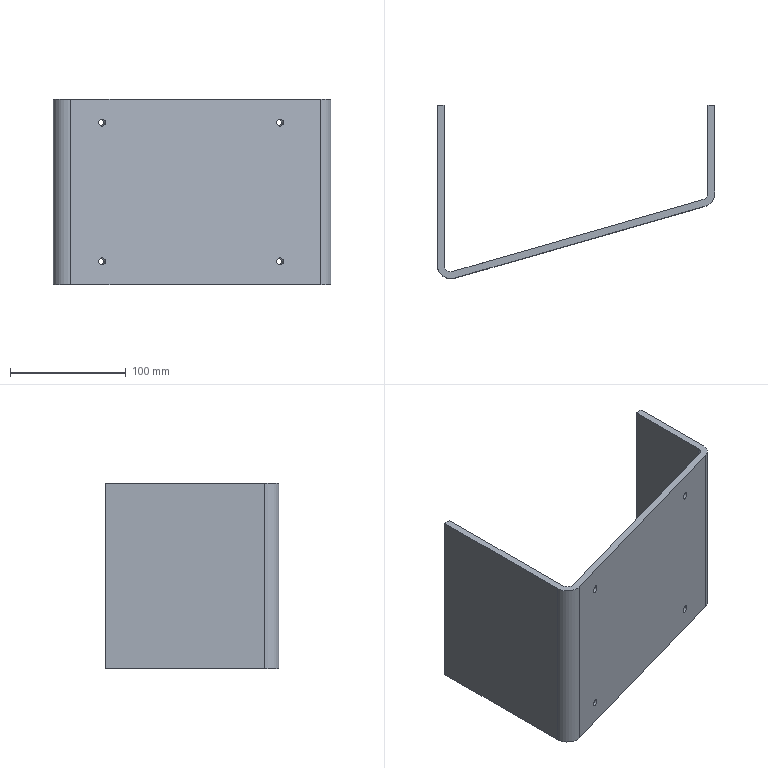Part | SolidWorks | features Extrusion 1, ICE 1 | 1 solid | 22 faces | box 240 x 149.894 x 160 mm | volume 447479 mm3 | cylinder 12 | plane 10 | commonest cylinder face diameters 6 x8 12 x2 24 x2
STEP:
#1=CARTESIAN_POINT('',(43.525,-135.096,20.));
#2=VERTEX_POINT('',#1);
#3=CARTESIAN_POINT('',(37.758,-136.75,20.));
#4=VERTEX_POINT('',#3);
#5=CARTESIAN_POINT('',(40.642,-135.923,20.));
#6=DIRECTION('',(-0.2756,0.9613,0.));
#7=DIRECTION('',(-0.9613,-0.2756,0.));
#8=AXIS2_PLACEMENT_3D('',#5,#6,#7);
#9=CIRCLE('',#8,3.);
#10=EDGE_CURVE('',#2,#4,#9,.T.);
#11=ORIENTED_EDGE('',*,*,#10,.T.);
#12=CARTESIAN_POINT('',(39.412,-142.518,20.));
#13=VERTEX_POINT('',#12);
#14=CARTESIAN_POINT('',(37.207,-134.828,20.));
#15=DIRECTION('',(0.2756,-0.9613,0.));
#16=VECTOR('',#15,1000.);
#17=LINE('',#14,#16);
#18=EDGE_CURVE('',#4,#13,#17,.T.);
#19=ORIENTED_EDGE('',*,*,#18,.T.);
#20=CARTESIAN_POINT('',(45.179,-140.864,20.));
#21=VERTEX_POINT('',#20);
#22=CARTESIAN_POINT('',(42.296,-141.691,20.));
#23=DIRECTION('',(0.2756,-0.9613,0.));
#24=DIRECTION('',(0.9613,0.2756,0.));
#25=AXIS2_PLACEMENT_3D('',#22,#23,#24);
#26=CIRCLE('',#25,3.);
#27=EDGE_CURVE('',#13,#21,#26,.T.);
#28=ORIENTED_EDGE('',*,*,#27,.T.);
#29=CARTESIAN_POINT('',(42.974,-133.174,20.));
#30=DIRECTION('',(0.2756,-0.9613,0.));
#31=VECTOR('',#30,1000.);
#32=LINE('',#29,#31);
#33=EDGE_CURVE('',#2,#21,#32,.T.);
#34=ORIENTED_EDGE('',*,*,#33,.F.);
#35=EDGE_LOOP('',(#11,#19,#28,#34));
#36=FACE_OUTER_BOUND('',#35,.T.);
#37=CARTESIAN_POINT('',(40.09,-134.001,20.));
#38=DIRECTION('',(0.2756,-0.9613,0.));
#39=DIRECTION('',(0.9613,0.2756,0.));
#40=AXIS2_PLACEMENT_3D('',#37,#38,#39);
#41=CYLINDRICAL_SURFACE('',#40,3.);
#42=ADVANCED_FACE('',(#36),#41,.F.);
#43=CARTESIAN_POINT('',(197.327,-90.994,140.));
#44=VERTEX_POINT('',#43);
#45=CARTESIAN_POINT('',(191.56,-92.648,140.));
#46=VERTEX_POINT('',#45);
#47=CARTESIAN_POINT('',(194.444,-91.821,140.));
#48=DIRECTION('',(-0.2756,0.9613,0.));
#49=DIRECTION('',(-0.9613,-0.2756,0.));
#50=AXIS2_PLACEMENT_3D('',#47,#48,#49);
#51=CIRCLE('',#50,3.);
#52=EDGE_CURVE('',#44,#46,#51,.T.);
#53=ORIENTED_EDGE('',*,*,#52,.T.);
#54=CARTESIAN_POINT('',(193.214,-98.416,140.));
#55=VERTEX_POINT('',#54);
#56=CARTESIAN_POINT('',(191.009,-90.726,140.));
#57=DIRECTION('',(0.2756,-0.9613,0.));
#58=VECTOR('',#57,1000.);
#59=LINE('',#56,#58);
#60=EDGE_CURVE('',#46,#55,#59,.T.);
#61=ORIENTED_EDGE('',*,*,#60,.T.);
#62=CARTESIAN_POINT('',(198.981,-96.762,140.));
#63=VERTEX_POINT('',#62);
#64=CARTESIAN_POINT('',(196.097,-97.589,140.));
#65=DIRECTION('',(0.2756,-0.9613,0.));
#66=DIRECTION('',(0.9613,0.2756,0.));
#67=AXIS2_PLACEMENT_3D('',#64,#65,#66);
#68=CIRCLE('',#67,3.);
#69=EDGE_CURVE('',#55,#63,#68,.T.);
#70=ORIENTED_EDGE('',*,*,#69,.T.);
#71=CARTESIAN_POINT('',(196.776,-89.072,140.));
#72=DIRECTION('',(0.2756,-0.9613,0.));
#73=VECTOR('',#72,1000.);
#74=LINE('',#71,#73);
#75=EDGE_CURVE('',#44,#63,#74,.T.);
#76=ORIENTED_EDGE('',*,*,#75,.F.);
#77=EDGE_LOOP('',(#53,#61,#70,#76));
#78=FACE_OUTER_BOUND('',#77,.T.);
#79=CARTESIAN_POINT('',(193.892,-89.899,140.));
#80=DIRECTION('',(0.2756,-0.9613,0.));
#81=DIRECTION('',(0.9613,0.2756,0.));
#82=AXIS2_PLACEMENT_3D('',#79,#80,#81);
#83=CYLINDRICAL_SURFACE('',#82,3.);
#84=ADVANCED_FACE('',(#78),#83,.F.);
#85=CARTESIAN_POINT('',(197.327,-90.994,20.));
#86=VERTEX_POINT('',#85);
#87=CARTESIAN_POINT('',(191.56,-92.648,20.));
#88=VERTEX_POINT('',#87);
#89=CARTESIAN_POINT('',(194.444,-91.821,20.));
#90=DIRECTION('',(-0.2756,0.9613,0.));
#91=DIRECTION('',(-0.9613,-0.2756,0.));
#92=AXIS2_PLACEMENT_3D('',#89,#90,#91);
#93=CIRCLE('',#92,3.);
#94=EDGE_CURVE('',#86,#88,#93,.T.);
#95=ORIENTED_EDGE('',*,*,#94,.T.);
#96=CARTESIAN_POINT('',(193.214,-98.416,20.));
#97=VERTEX_POINT('',#96);
#98=CARTESIAN_POINT('',(191.009,-90.726,20.));
#99=DIRECTION('',(0.2756,-0.9613,0.));
#100=VECTOR('',#99,1000.);
#101=LINE('',#98,#100);
#102=EDGE_CURVE('',#88,#97,#101,.T.);
#103=ORIENTED_EDGE('',*,*,#102,.T.);
#104=CARTESIAN_POINT('',(198.981,-96.762,20.));
#105=VERTEX_POINT('',#104);
#106=CARTESIAN_POINT('',(196.097,-97.589,20.));
#107=DIRECTION('',(0.2756,-0.9613,0.));
#108=DIRECTION('',(0.9613,0.2756,0.));
#109=AXIS2_PLACEMENT_3D('',#106,#107,#108);
#110=CIRCLE('',#109,3.);
#111=EDGE_CURVE('',#97,#105,#110,.T.);
#112=ORIENTED_EDGE('',*,*,#111,.T.);
#113=CARTESIAN_POINT('',(196.776,-89.072,20.));
#114=DIRECTION('',(0.2756,-0.9613,0.));
#115=VECTOR('',#114,1000.);
#116=LINE('',#113,#115);
#117=EDGE_CURVE('',#86,#105,#116,.T.);
#118=ORIENTED_EDGE('',*,*,#117,.F.);
#119=EDGE_LOOP('',(#95,#103,#112,#118));
#120=FACE_OUTER_BOUND('',#119,.T.);
#121=CARTESIAN_POINT('',(193.892,-89.899,20.));
#122=DIRECTION('',(0.2756,-0.9613,0.));
#123=DIRECTION('',(0.9613,0.2756,0.));
#124=AXIS2_PLACEMENT_3D('',#121,#122,#123);
#125=CYLINDRICAL_SURFACE('',#124,3.);
#126=ADVANCED_FACE('',(#120),#125,.F.);
#127=CARTESIAN_POINT('',(43.525,-135.096,140.));
#128=VERTEX_POINT('',#127);
#129=CARTESIAN_POINT('',(37.758,-136.75,140.));
#130=VERTEX_POINT('',#129);
#131=CARTESIAN_POINT('',(40.642,-135.923,140.));
#132=DIRECTION('',(-0.2756,0.9613,0.));
#133=DIRECTION('',(-0.9613,-0.2756,0.));
#134=AXIS2_PLACEMENT_3D('',#131,#132,#133);
#135=CIRCLE('',#134,3.);
#136=EDGE_CURVE('',#128,#130,#135,.T.);
#137=ORIENTED_EDGE('',*,*,#136,.T.);
#138=CARTESIAN_POINT('',(39.412,-142.518,140.));
#139=VERTEX_POINT('',#138);
#140=CARTESIAN_POINT('',(37.207,-134.828,140.));
#141=DIRECTION('',(0.2756,-0.9613,0.));
#142=VECTOR('',#141,1000.);
#143=LINE('',#140,#142);
#144=EDGE_CURVE('',#130,#139,#143,.T.);
#145=ORIENTED_EDGE('',*,*,#144,.T.);
#146=CARTESIAN_POINT('',(45.179,-140.864,140.));
#147=VERTEX_POINT('',#146);
#148=CARTESIAN_POINT('',(42.296,-141.691,140.));
#149=DIRECTION('',(0.2756,-0.9613,0.));
#150=DIRECTION('',(0.9613,0.2756,0.));
#151=AXIS2_PLACEMENT_3D('',#148,#149,#150);
#152=CIRCLE('',#151,3.);
#153=EDGE_CURVE('',#139,#147,#152,.T.);
#154=ORIENTED_EDGE('',*,*,#153,.T.);
#155=CARTESIAN_POINT('',(42.974,-133.174,140.));
#156=DIRECTION('',(0.2756,-0.9613,0.));
#157=VECTOR('',#156,1000.);
#158=LINE('',#155,#157);
#159=EDGE_CURVE('',#128,#147,#158,.T.);
#160=ORIENTED_EDGE('',*,*,#159,.F.);
#161=EDGE_LOOP('',(#137,#145,#154,#160));
#162=FACE_OUTER_BOUND('',#161,.T.);
#163=CARTESIAN_POINT('',(40.09,-134.001,140.));
#164=DIRECTION('',(0.2756,-0.9613,0.));
#165=DIRECTION('',(0.9613,0.2756,0.));
#166=AXIS2_PLACEMENT_3D('',#163,#164,#165);
#167=CYLINDRICAL_SURFACE('',#166,3.);
#168=ADVANCED_FACE('',(#162),#167,.F.);
#169=CARTESIAN_POINT('',(234.,-75.957,0.));
#170=VERTEX_POINT('',#169);
#171=CARTESIAN_POINT('',(234.,0.,0.));
#172=VERTEX_POINT('',#171);
#173=CARTESIAN_POINT('',(234.,-75.957,0.));
#174=DIRECTION('',(0.,1.,0.));
#175=VECTOR('',#174,1000.);
#176=LINE('',#173,#175);
#177=EDGE_CURVE('',#170,#172,#176,.T.);
#178=ORIENTED_EDGE('',*,*,#177,.F.);
#179=CARTESIAN_POINT('',(234.,-75.957,160.));
#180=VERTEX_POINT('',#179);
#181=CARTESIAN_POINT('',(234.,-75.957,160.));
#182=DIRECTION('',(0.,0.,-1.));
#183=VECTOR('',#182,1000.);
#184=LINE('',#181,#183);
#185=EDGE_CURVE('',#180,#170,#184,.T.);
#186=ORIENTED_EDGE('',*,*,#185,.F.);
#187=CARTESIAN_POINT('',(234.,0.,160.));
#188=VERTEX_POINT('',#187);
#189=CARTESIAN_POINT('',(234.,-75.957,160.));
#190=DIRECTION('',(0.,1.,0.));
#191=VECTOR('',#190,1000.);
#192=LINE('',#189,#191);
#193=EDGE_CURVE('',#180,#188,#192,.T.);
#194=ORIENTED_EDGE('',*,*,#193,.T.);
#195=CARTESIAN_POINT('',(234.,0.,160.));
#196=DIRECTION('',(0.,0.,-1.));
#197=VECTOR('',#196,1000.);
#198=LINE('',#195,#197);
#199=EDGE_CURVE('',#188,#172,#198,.T.);
#200=ORIENTED_EDGE('',*,*,#199,.T.);
#201=EDGE_LOOP('',(#178,#186,#194,#200));
#202=FACE_OUTER_BOUND('',#201,.T.);
#203=CARTESIAN_POINT('',(234.,-75.957,160.));
#204=DIRECTION('',(-1.,0.,0.));
#205=DIRECTION('',(0.,-1.,0.));
#206=AXIS2_PLACEMENT_3D('',#203,#204,#205);
#207=PLANE('',#206);
#208=ADVANCED_FACE('',(#202),#207,.T.);
#209=CARTESIAN_POINT('',(229.654,-81.725,0.));
#210=VERTEX_POINT('',#209);
#211=CARTESIAN_POINT('',(228.,-75.957,0.));
#212=DIRECTION('',(0.,0.,1.));
#213=DIRECTION('',(1.,0.,0.));
#214=AXIS2_PLACEMENT_3D('',#211,#212,#213);
#215=CIRCLE('',#214,6.);
#216=EDGE_CURVE('',#210,#170,#215,.T.);
#217=ORIENTED_EDGE('',*,*,#216,.F.);
#218=CARTESIAN_POINT('',(229.654,-81.725,160.));
#219=VERTEX_POINT('',#218);
#220=CARTESIAN_POINT('',(229.654,-81.725,160.));
#221=DIRECTION('',(0.,0.,-1.));
#222=VECTOR('',#221,1000.);
#223=LINE('',#220,#222);
#224=EDGE_CURVE('',#219,#210,#223,.T.);
#225=ORIENTED_EDGE('',*,*,#224,.F.);
#226=CARTESIAN_POINT('',(228.,-75.957,160.));
#227=DIRECTION('',(0.,0.,1.));
#228=DIRECTION('',(1.,0.,0.));
#229=AXIS2_PLACEMENT_3D('',#226,#227,#228);
#230=CIRCLE('',#229,6.);
#231=EDGE_CURVE('',#219,#180,#230,.T.);
#232=ORIENTED_EDGE('',*,*,#231,.T.);
#233=ORIENTED_EDGE('',*,*,#185,.T.);
#234=EDGE_LOOP('',(#217,#225,#232,#233));
#235=FACE_OUTER_BOUND('',#234,.T.);
#236=CARTESIAN_POINT('',(228.,-75.957,160.));
#237=DIRECTION('',(0.,0.,-1.));
#238=DIRECTION('',(-1.,0.,0.));
#239=AXIS2_PLACEMENT_3D('',#236,#237,#238);
#240=CYLINDRICAL_SURFACE('',#239,6.);
#241=ADVANCED_FACE('',(#235),#240,.F.);
#242=ORIENTED_EDGE('',*,*,#10,.F.);
#243=CARTESIAN_POINT('',(40.642,-135.923,20.));
#244=DIRECTION('',(-0.2756,0.9613,0.));
#245=DIRECTION('',(-0.9613,-0.2756,0.));
#246=AXIS2_PLACEMENT_3D('',#243,#244,#245);
#247=CIRCLE('',#246,3.);
#248=EDGE_CURVE('',#4,#2,#247,.T.);
#249=ORIENTED_EDGE('',*,*,#248,.F.);
#250=EDGE_LOOP('',(#242,#249));
#251=FACE_BOUND('',#250,.T.);
#252=ORIENTED_EDGE('',*,*,#52,.F.);
#253=CARTESIAN_POINT('',(194.444,-91.821,140.));
#254=DIRECTION('',(-0.2756,0.9613,0.));
#255=DIRECTION('',(-0.9613,-0.2756,0.));
#256=AXIS2_PLACEMENT_3D('',#253,#254,#255);
#257=CIRCLE('',#256,3.);
#258=EDGE_CURVE('',#46,#44,#257,.T.);
#259=ORIENTED_EDGE('',*,*,#258,.F.);
#260=EDGE_LOOP('',(#252,#259));
#261=FACE_BOUND('',#260,.T.);
#262=ORIENTED_EDGE('',*,*,#94,.F.);
#263=CARTESIAN_POINT('',(194.444,-91.821,20.));
#264=DIRECTION('',(-0.2756,0.9613,0.));
#265=DIRECTION('',(-0.9613,-0.2756,0.));
#266=AXIS2_PLACEMENT_3D('',#263,#264,#265);
#267=CIRCLE('',#266,3.);
#268=EDGE_CURVE('',#88,#86,#267,.T.);
#269=ORIENTED_EDGE('',*,*,#268,.F.);
#270=EDGE_LOOP('',(#262,#269));
#271=FACE_BOUND('',#270,.T.);
#272=ORIENTED_EDGE('',*,*,#136,.F.);
#273=CARTESIAN_POINT('',(40.642,-135.923,140.));
#274=DIRECTION('',(-0.2756,0.9613,0.));
#275=DIRECTION('',(-0.9613,-0.2756,0.));
#276=AXIS2_PLACEMENT_3D('',#273,#274,#275);
#277=CIRCLE('',#276,3.);
#278=EDGE_CURVE('',#130,#128,#277,.T.);
#279=ORIENTED_EDGE('',*,*,#278,.F.);
#280=EDGE_LOOP('',(#272,#279));
#281=FACE_BOUND('',#280,.T.);
#282=CARTESIAN_POINT('',(13.654,-143.662,0.));
#283=VERTEX_POINT('',#282);
#284=CARTESIAN_POINT('',(13.654,-143.662,0.));
#285=DIRECTION('',(0.9613,0.2756,0.));
#286=VECTOR('',#285,1000.);
#287=LINE('',#284,#286);
#288=EDGE_CURVE('',#283,#210,#287,.T.);
#289=ORIENTED_EDGE('',*,*,#288,.F.);
#290=CARTESIAN_POINT('',(13.654,-143.662,160.));
#291=VERTEX_POINT('',#290);
#292=CARTESIAN_POINT('',(13.654,-143.662,160.));
#293=DIRECTION('',(0.,0.,-1.));
#294=VECTOR('',#293,1000.);
#295=LINE('',#292,#294);
#296=EDGE_CURVE('',#291,#283,#295,.T.);
#297=ORIENTED_EDGE('',*,*,#296,.F.);
#298=CARTESIAN_POINT('',(13.654,-143.662,160.));
#299=DIRECTION('',(0.9613,0.2756,0.));
#300=VECTOR('',#299,1000.);
#301=LINE('',#298,#300);
#302=EDGE_CURVE('',#291,#219,#301,.T.);
#303=ORIENTED_EDGE('',*,*,#302,.T.);
#304=ORIENTED_EDGE('',*,*,#224,.T.);
#305=EDGE_LOOP('',(#289,#297,#303,#304));
#306=FACE_OUTER_BOUND('',#305,.T.);
#307=CARTESIAN_POINT('',(13.654,-143.662,160.));
#308=DIRECTION('',(-0.2756,0.9613,0.));
#309=DIRECTION('',(-0.9613,-0.2756,0.));
#310=AXIS2_PLACEMENT_3D('',#307,#308,#309);
#311=PLANE('',#310);
#312=ADVANCED_FACE('',(#251,#261,#271,#281,#306),#311,.T.);
#313=CARTESIAN_POINT('',(6.,-137.894,0.));
#314=VERTEX_POINT('',#313);
#315=CARTESIAN_POINT('',(12.,-137.894,0.));
#316=DIRECTION('',(0.,0.,1.));
#317=DIRECTION('',(1.,0.,0.));
#318=AXIS2_PLACEMENT_3D('',#315,#316,#317);
#319=CIRCLE('',#318,6.);
#320=EDGE_CURVE('',#314,#283,#319,.T.);
#321=ORIENTED_EDGE('',*,*,#320,.F.);
#322=CARTESIAN_POINT('',(6.,-137.894,160.));
#323=VERTEX_POINT('',#322);
#324=CARTESIAN_POINT('',(6.,-137.894,160.));
#325=DIRECTION('',(0.,0.,-1.));
#326=VECTOR('',#325,1000.);
#327=LINE('',#324,#326);
#328=EDGE_CURVE('',#323,#314,#327,.T.);
#329=ORIENTED_EDGE('',*,*,#328,.F.);
#330=CARTESIAN_POINT('',(12.,-137.894,160.));
#331=DIRECTION('',(0.,0.,1.));
#332=DIRECTION('',(1.,0.,0.));
#333=AXIS2_PLACEMENT_3D('',#330,#331,#332);
#334=CIRCLE('',#333,6.);
#335=EDGE_CURVE('',#323,#291,#334,.T.);
#336=ORIENTED_EDGE('',*,*,#335,.T.);
#337=ORIENTED_EDGE('',*,*,#296,.T.);
#338=EDGE_LOOP('',(#321,#329,#336,#337));
#339=FACE_OUTER_BOUND('',#338,.T.);
#340=CARTESIAN_POINT('',(12.,-137.894,160.));
#341=DIRECTION('',(0.,0.,-1.));
#342=DIRECTION('',(-1.,0.,0.));
#343=AXIS2_PLACEMENT_3D('',#340,#341,#342);
#344=CYLINDRICAL_SURFACE('',#343,6.);
#345=ADVANCED_FACE('',(#339),#344,.F.);
#346=CARTESIAN_POINT('',(6.,0.,0.));
#347=VERTEX_POINT('',#346);
#348=CARTESIAN_POINT('',(6.,0.,0.));
#349=DIRECTION('',(0.,-1.,0.));
#350=VECTOR('',#349,1000.);
#351=LINE('',#348,#350);
#352=EDGE_CURVE('',#347,#314,#351,.T.);
#353=ORIENTED_EDGE('',*,*,#352,.F.);
#354=CARTESIAN_POINT('',(6.,0.,160.));
#355=VERTEX_POINT('',#354);
#356=CARTESIAN_POINT('',(6.,0.,160.));
#357=DIRECTION('',(0.,0.,-1.));
#358=VECTOR('',#357,1000.);
#359=LINE('',#356,#358);
#360=EDGE_CURVE('',#355,#347,#359,.T.);
#361=ORIENTED_EDGE('',*,*,#360,.F.);
#362=CARTESIAN_POINT('',(6.,0.,160.));
#363=DIRECTION('',(0.,-1.,0.));
#364=VECTOR('',#363,1000.);
#365=LINE('',#362,#364);
#366=EDGE_CURVE('',#355,#323,#365,.T.);
#367=ORIENTED_EDGE('',*,*,#366,.T.);
#368=ORIENTED_EDGE('',*,*,#328,.T.);
#369=EDGE_LOOP('',(#353,#361,#367,#368));
#370=FACE_OUTER_BOUND('',#369,.T.);
#371=CARTESIAN_POINT('',(6.,0.,160.));
#372=DIRECTION('',(1.,0.,0.));
#373=DIRECTION('',(0.,1.,0.));
#374=AXIS2_PLACEMENT_3D('',#371,#372,#373);
#375=PLANE('',#374);
#376=ADVANCED_FACE('',(#370),#375,.T.);
#377=CARTESIAN_POINT('',(0.,0.,0.));
#378=VERTEX_POINT('',#377);
#379=CARTESIAN_POINT('',(6.,0.,0.));
#380=DIRECTION('',(-1.,0.,0.));
#381=VECTOR('',#380,1000.);
#382=LINE('',#379,#381);
#383=EDGE_CURVE('',#347,#378,#382,.T.);
#384=ORIENTED_EDGE('',*,*,#383,.T.);
#385=CARTESIAN_POINT('',(0.,0.,160.));
#386=VERTEX_POINT('',#385);
#387=CARTESIAN_POINT('',(0.,0.,160.));
#388=DIRECTION('',(0.,0.,-1.));
#389=VECTOR('',#388,1000.);
#390=LINE('',#387,#389);
#391=EDGE_CURVE('',#386,#378,#390,.T.);
#392=ORIENTED_EDGE('',*,*,#391,.F.);
#393=CARTESIAN_POINT('',(6.,0.,160.));
#394=DIRECTION('',(-1.,0.,0.));
#395=VECTOR('',#394,1000.);
#396=LINE('',#393,#395);
#397=EDGE_CURVE('',#355,#386,#396,.T.);
#398=ORIENTED_EDGE('',*,*,#397,.F.);
#399=ORIENTED_EDGE('',*,*,#360,.T.);
#400=EDGE_LOOP('',(#384,#392,#398,#399));
#401=FACE_OUTER_BOUND('',#400,.T.);
#402=CARTESIAN_POINT('',(6.,0.,160.));
#403=DIRECTION('',(0.,-1.,0.));
#404=DIRECTION('',(0.,0.,-1.));
#405=AXIS2_PLACEMENT_3D('',#402,#403,#404);
#406=PLANE('',#405);
#407=ADVANCED_FACE('',(#401),#406,.F.);
#408=CARTESIAN_POINT('',(0.,-137.894,0.));
#409=VERTEX_POINT('',#408);
#410=CARTESIAN_POINT('',(0.,0.,0.));
#411=DIRECTION('',(0.,-1.,0.));
#412=VECTOR('',#411,1000.);
#413=LINE('',#410,#412);
#414=EDGE_CURVE('',#378,#409,#413,.T.);
#415=ORIENTED_EDGE('',*,*,#414,.T.);
#416=CARTESIAN_POINT('',(0.,-137.894,160.));
#417=VERTEX_POINT('',#416);
#418=CARTESIAN_POINT('',(0.,-137.894,160.));
#419=DIRECTION('',(0.,0.,-1.));
#420=VECTOR('',#419,1000.);
#421=LINE('',#418,#420);
#422=EDGE_CURVE('',#417,#409,#421,.T.);
#423=ORIENTED_EDGE('',*,*,#422,.F.);
#424=CARTESIAN_POINT('',(0.,0.,160.));
#425=DIRECTION('',(0.,-1.,0.));
#426=VECTOR('',#425,1000.);
#427=LINE('',#424,#426);
#428=EDGE_CURVE('',#386,#417,#427,.T.);
#429=ORIENTED_EDGE('',*,*,#428,.F.);
#430=ORIENTED_EDGE('',*,*,#391,.T.);
#431=EDGE_LOOP('',(#415,#423,#429,#430));
#432=FACE_OUTER_BOUND('',#431,.T.);
#433=CARTESIAN_POINT('',(0.,0.,160.));
#434=DIRECTION('',(1.,0.,0.));
#435=DIRECTION('',(0.,1.,0.));
#436=AXIS2_PLACEMENT_3D('',#433,#434,#435);
#437=PLANE('',#436);
#438=ADVANCED_FACE('',(#432),#437,.F.);
#439=CARTESIAN_POINT('',(15.308,-149.429,0.));
#440=VERTEX_POINT('',#439);
#441=CARTESIAN_POINT('',(12.,-137.894,0.));
#442=DIRECTION('',(0.,0.,1.));
#443=DIRECTION('',(1.,0.,0.));
#444=AXIS2_PLACEMENT_3D('',#441,#442,#443);
#445=CIRCLE('',#444,12.);
#446=EDGE_CURVE('',#409,#440,#445,.T.);
#447=ORIENTED_EDGE('',*,*,#446,.T.);
#448=CARTESIAN_POINT('',(15.308,-149.429,160.));
#449=VERTEX_POINT('',#448);
#450=CARTESIAN_POINT('',(15.308,-149.429,160.));
#451=DIRECTION('',(0.,0.,-1.));
#452=VECTOR('',#451,1000.);
#453=LINE('',#450,#452);
#454=EDGE_CURVE('',#449,#440,#453,.T.);
#455=ORIENTED_EDGE('',*,*,#454,.F.);
#456=CARTESIAN_POINT('',(12.,-137.894,160.));
#457=DIRECTION('',(0.,0.,1.));
#458=DIRECTION('',(1.,0.,0.));
#459=AXIS2_PLACEMENT_3D('',#456,#457,#458);
#460=CIRCLE('',#459,12.);
#461=EDGE_CURVE('',#417,#449,#460,.T.);
#462=ORIENTED_EDGE('',*,*,#461,.F.);
#463=ORIENTED_EDGE('',*,*,#422,.T.);
#464=EDGE_LOOP('',(#447,#455,#462,#463));
#465=FACE_OUTER_BOUND('',#464,.T.);
#466=CARTESIAN_POINT('',(12.,-137.894,160.));
#467=DIRECTION('',(0.,0.,-1.));
#468=DIRECTION('',(-1.,0.,0.));
#469=AXIS2_PLACEMENT_3D('',#466,#467,#468);
#470=CYLINDRICAL_SURFACE('',#469,12.);
#471=ADVANCED_FACE('',(#465),#470,.T.);
#472=CARTESIAN_POINT('',(42.296,-141.691,20.));
#473=DIRECTION('',(0.2756,-0.9613,0.));
#474=DIRECTION('',(0.9613,0.2756,0.));
#475=AXIS2_PLACEMENT_3D('',#472,#473,#474);
#476=CIRCLE('',#475,3.);
#477=EDGE_CURVE('',#21,#13,#476,.T.);
#478=ORIENTED_EDGE('',*,*,#477,.F.);
#479=ORIENTED_EDGE('',*,*,#27,.F.);
#480=EDGE_LOOP('',(#478,#479));
#481=FACE_BOUND('',#480,.T.);
#482=CARTESIAN_POINT('',(196.097,-97.589,140.));
#483=DIRECTION('',(0.2756,-0.9613,0.));
#484=DIRECTION('',(0.9613,0.2756,0.));
#485=AXIS2_PLACEMENT_3D('',#482,#483,#484);
#486=CIRCLE('',#485,3.);
#487=EDGE_CURVE('',#63,#55,#486,.T.);
#488=ORIENTED_EDGE('',*,*,#487,.F.);
#489=ORIENTED_EDGE('',*,*,#69,.F.);
#490=EDGE_LOOP('',(#488,#489));
#491=FACE_BOUND('',#490,.T.);
#492=CARTESIAN_POINT('',(196.097,-97.589,20.));
#493=DIRECTION('',(0.2756,-0.9613,0.));
#494=DIRECTION('',(0.9613,0.2756,0.));
#495=AXIS2_PLACEMENT_3D('',#492,#493,#494);
#496=CIRCLE('',#495,3.);
#497=EDGE_CURVE('',#105,#97,#496,.T.);
#498=ORIENTED_EDGE('',*,*,#497,.F.);
#499=ORIENTED_EDGE('',*,*,#111,.F.);
#500=EDGE_LOOP('',(#498,#499));
#501=FACE_BOUND('',#500,.T.);
#502=CARTESIAN_POINT('',(42.296,-141.691,140.));
#503=DIRECTION('',(0.2756,-0.9613,0.));
#504=DIRECTION('',(0.9613,0.2756,0.));
#505=AXIS2_PLACEMENT_3D('',#502,#503,#504);
#506=CIRCLE('',#505,3.);
#507=EDGE_CURVE('',#147,#139,#506,.T.);
#508=ORIENTED_EDGE('',*,*,#507,.F.);
#509=ORIENTED_EDGE('',*,*,#153,.F.);
#510=EDGE_LOOP('',(#508,#509));
#511=FACE_BOUND('',#510,.T.);
#512=CARTESIAN_POINT('',(231.308,-87.492,0.));
#513=VERTEX_POINT('',#512);
#514=CARTESIAN_POINT('',(15.308,-149.429,0.));
#515=DIRECTION('',(0.9613,0.2756,0.));
#516=VECTOR('',#515,1000.);
#517=LINE('',#514,#516);
#518=EDGE_CURVE('',#440,#513,#517,.T.);
#519=ORIENTED_EDGE('',*,*,#518,.T.);
#520=CARTESIAN_POINT('',(231.308,-87.492,160.));
#521=VERTEX_POINT('',#520);
#522=CARTESIAN_POINT('',(231.308,-87.492,160.));
#523=DIRECTION('',(0.,0.,-1.));
#524=VECTOR('',#523,1000.);
#525=LINE('',#522,#524);
#526=EDGE_CURVE('',#521,#513,#525,.T.);
#527=ORIENTED_EDGE('',*,*,#526,.F.);
#528=CARTESIAN_POINT('',(15.308,-149.429,160.));
#529=DIRECTION('',(0.9613,0.2756,0.));
#530=VECTOR('',#529,1000.);
#531=LINE('',#528,#530);
#532=EDGE_CURVE('',#449,#521,#531,.T.);
#533=ORIENTED_EDGE('',*,*,#532,.F.);
#534=ORIENTED_EDGE('',*,*,#454,.T.);
#535=EDGE_LOOP('',(#519,#527,#533,#534));
#536=FACE_OUTER_BOUND('',#535,.T.);
#537=CARTESIAN_POINT('',(15.308,-149.429,160.));
#538=DIRECTION('',(-0.2756,0.9613,0.));
#539=DIRECTION('',(-0.9613,-0.2756,0.));
#540=AXIS2_PLACEMENT_3D('',#537,#538,#539);
#541=PLANE('',#540);
#542=ADVANCED_FACE('',(#481,#491,#501,#511,#536),#541,.F.);
#543=CARTESIAN_POINT('',(240.,-75.957,0.));
#544=VERTEX_POINT('',#543);
#545=CARTESIAN_POINT('',(228.,-75.957,0.));
#546=DIRECTION('',(0.,0.,1.));
#547=DIRECTION('',(1.,0.,0.));
#548=AXIS2_PLACEMENT_3D('',#545,#546,#547);
#549=CIRCLE('',#548,12.);
#550=EDGE_CURVE('',#513,#544,#549,.T.);
#551=ORIENTED_EDGE('',*,*,#550,.T.);
#552=CARTESIAN_POINT('',(240.,-75.957,160.));
#553=VERTEX_POINT('',#552);
#554=CARTESIAN_POINT('',(240.,-75.957,160.));
#555=DIRECTION('',(0.,0.,-1.));
#556=VECTOR('',#555,1000.);
#557=LINE('',#554,#556);
#558=EDGE_CURVE('',#553,#544,#557,.T.);
#559=ORIENTED_EDGE('',*,*,#558,.F.);
#560=CARTESIAN_POINT('',(228.,-75.957,160.));
#561=DIRECTION('',(0.,0.,1.));
#562=DIRECTION('',(1.,0.,0.));
#563=AXIS2_PLACEMENT_3D('',#560,#561,#562);
#564=CIRCLE('',#563,12.);
#565=EDGE_CURVE('',#521,#553,#564,.T.);
#566=ORIENTED_EDGE('',*,*,#565,.F.);
#567=ORIENTED_EDGE('',*,*,#526,.T.);
#568=EDGE_LOOP('',(#551,#559,#566,#567));
#569=FACE_OUTER_BOUND('',#568,.T.);
#570=CARTESIAN_POINT('',(228.,-75.957,160.));
#571=DIRECTION('',(0.,0.,-1.));
#572=DIRECTION('',(-1.,0.,0.));
#573=AXIS2_PLACEMENT_3D('',#570,#571,#572);
#574=CYLINDRICAL_SURFACE('',#573,12.);
#575=ADVANCED_FACE('',(#569),#574,.T.);
#576=CARTESIAN_POINT('',(240.,0.,0.));
#577=VERTEX_POINT('',#576);
#578=CARTESIAN_POINT('',(240.,-75.957,0.));
#579=DIRECTION('',(0.,1.,0.));
#580=VECTOR('',#579,1000.);
#581=LINE('',#578,#580);
#582=EDGE_CURVE('',#544,#577,#581,.T.);
#583=ORIENTED_EDGE('',*,*,#582,.T.);
#584=CARTESIAN_POINT('',(240.,0.,160.));
#585=VERTEX_POINT('',#584);
#586=CARTESIAN_POINT('',(240.,0.,160.));
#587=DIRECTION('',(0.,0.,-1.));
#588=VECTOR('',#587,1000.);
#589=LINE('',#586,#588);
#590=EDGE_CURVE('',#585,#577,#589,.T.);
#591=ORIENTED_EDGE('',*,*,#590,.F.);
#592=CARTESIAN_POINT('',(240.,-75.957,160.));
#593=DIRECTION('',(0.,1.,0.));
#594=VECTOR('',#593,1000.);
#595=LINE('',#592,#594);
#596=EDGE_CURVE('',#553,#585,#595,.T.);
#597=ORIENTED_EDGE('',*,*,#596,.F.);
#598=ORIENTED_EDGE('',*,*,#558,.T.);
#599=EDGE_LOOP('',(#583,#591,#597,#598));
#600=FACE_OUTER_BOUND('',#599,.T.);
#601=CARTESIAN_POINT('',(240.,-75.957,160.));
#602=DIRECTION('',(-1.,0.,0.));
#603=DIRECTION('',(0.,0.,1.));
#604=AXIS2_PLACEMENT_3D('',#601,#602,#603);
#605=PLANE('',#604);
#606=ADVANCED_FACE('',(#600),#605,.F.);
#607=CARTESIAN_POINT('',(234.,0.,0.));
#608=DIRECTION('',(1.,0.,0.));
#609=VECTOR('',#608,1000.);
#610=LINE('',#607,#609);
#611=EDGE_CURVE('',#172,#577,#610,.T.);
#612=ORIENTED_EDGE('',*,*,#611,.F.);
#613=ORIENTED_EDGE('',*,*,#199,.F.);
#614=CARTESIAN_POINT('',(234.,0.,160.));
#615=DIRECTION('',(1.,0.,0.));
#616=VECTOR('',#615,1000.);
#617=LINE('',#614,#616);
#618=EDGE_CURVE('',#188,#585,#617,.T.);
#619=ORIENTED_EDGE('',*,*,#618,.T.);
#620=ORIENTED_EDGE('',*,*,#590,.T.);
#621=EDGE_LOOP('',(#612,#613,#619,#620));
#622=FACE_OUTER_BOUND('',#621,.T.);
#623=CARTESIAN_POINT('',(234.,0.,160.));
#624=DIRECTION('',(0.,1.,0.));
#625=DIRECTION('',(-1.,0.,0.));
#626=AXIS2_PLACEMENT_3D('',#623,#624,#625);
#627=PLANE('',#626);
#628=ADVANCED_FACE('',(#622),#627,.T.);
#629=ORIENTED_EDGE('',*,*,#193,.F.);
#630=ORIENTED_EDGE('',*,*,#231,.F.);
#631=ORIENTED_EDGE('',*,*,#302,.F.);
#632=ORIENTED_EDGE('',*,*,#335,.F.);
#633=ORIENTED_EDGE('',*,*,#366,.F.);
#634=ORIENTED_EDGE('',*,*,#397,.T.);
#635=ORIENTED_EDGE('',*,*,#428,.T.);
#636=ORIENTED_EDGE('',*,*,#461,.T.);
#637=ORIENTED_EDGE('',*,*,#532,.T.);
#638=ORIENTED_EDGE('',*,*,#565,.T.);
#639=ORIENTED_EDGE('',*,*,#596,.T.);
#640=ORIENTED_EDGE('',*,*,#618,.F.);
#641=EDGE_LOOP('',(#629,#630,#631,#632,#633,#634,#635,#636,#637,#638,#639,#640));
#642=FACE_OUTER_BOUND('',#641,.T.);
#643=CARTESIAN_POINT('',(228.,-75.957,160.));
#644=DIRECTION('',(0.,0.,1.));
#645=DIRECTION('',(1.,0.,0.));
#646=AXIS2_PLACEMENT_3D('',#643,#644,#645);
#647=PLANE('',#646);
#648=ADVANCED_FACE('',(#642),#647,.T.);
#649=ORIENTED_EDGE('',*,*,#177,.T.);
#650=ORIENTED_EDGE('',*,*,#611,.T.);
#651=ORIENTED_EDGE('',*,*,#582,.F.);
#652=ORIENTED_EDGE('',*,*,#550,.F.);
#653=ORIENTED_EDGE('',*,*,#518,.F.);
#654=ORIENTED_EDGE('',*,*,#446,.F.);
#655=ORIENTED_EDGE('',*,*,#414,.F.);
#656=ORIENTED_EDGE('',*,*,#383,.F.);
#657=ORIENTED_EDGE('',*,*,#352,.T.);
#658=ORIENTED_EDGE('',*,*,#320,.T.);
#659=ORIENTED_EDGE('',*,*,#288,.T.);
#660=ORIENTED_EDGE('',*,*,#216,.T.);
#661=EDGE_LOOP('',(#649,#650,#651,#652,#653,#654,#655,#656,#657,#658,#659,#660));
#662=FACE_OUTER_BOUND('',#661,.T.);
#663=CARTESIAN_POINT('',(228.,-75.957,0.));
#664=DIRECTION('',(0.,0.,1.));
#665=DIRECTION('',(1.,0.,0.));
#666=AXIS2_PLACEMENT_3D('',#663,#664,#665);
#667=PLANE('',#666);
#668=ADVANCED_FACE('',(#662),#667,.F.);
#669=ORIENTED_EDGE('',*,*,#144,.F.);
#670=ORIENTED_EDGE('',*,*,#278,.T.);
#671=ORIENTED_EDGE('',*,*,#159,.T.);
#672=ORIENTED_EDGE('',*,*,#507,.T.);
#673=EDGE_LOOP('',(#669,#670,#671,#672));
#674=FACE_OUTER_BOUND('',#673,.T.);
#675=CARTESIAN_POINT('',(40.09,-134.001,140.));
#676=DIRECTION('',(0.2756,-0.9613,0.));
#677=DIRECTION('',(0.9613,0.2756,0.));
#678=AXIS2_PLACEMENT_3D('',#675,#676,#677);
#679=CYLINDRICAL_SURFACE('',#678,3.);
#680=ADVANCED_FACE('',(#674),#679,.F.);
#681=ORIENTED_EDGE('',*,*,#102,.F.);
#682=ORIENTED_EDGE('',*,*,#268,.T.);
#683=ORIENTED_EDGE('',*,*,#117,.T.);
#684=ORIENTED_EDGE('',*,*,#497,.T.);
#685=EDGE_LOOP('',(#681,#682,#683,#684));
#686=FACE_OUTER_BOUND('',#685,.T.);
#687=CARTESIAN_POINT('',(193.892,-89.899,20.));
#688=DIRECTION('',(0.2756,-0.9613,0.));
#689=DIRECTION('',(0.9613,0.2756,0.));
#690=AXIS2_PLACEMENT_3D('',#687,#688,#689);
#691=CYLINDRICAL_SURFACE('',#690,3.);
#692=ADVANCED_FACE('',(#686),#691,.F.);
#693=ORIENTED_EDGE('',*,*,#60,.F.);
#694=ORIENTED_EDGE('',*,*,#258,.T.);
#695=ORIENTED_EDGE('',*,*,#75,.T.);
#696=ORIENTED_EDGE('',*,*,#487,.T.);
#697=EDGE_LOOP('',(#693,#694,#695,#696));
#698=FACE_OUTER_BOUND('',#697,.T.);
#699=CARTESIAN_POINT('',(193.892,-89.899,140.));
#700=DIRECTION('',(0.2756,-0.9613,0.));
#701=DIRECTION('',(0.9613,0.2756,0.));
#702=AXIS2_PLACEMENT_3D('',#699,#700,#701);
#703=CYLINDRICAL_SURFACE('',#702,3.);
#704=ADVANCED_FACE('',(#698),#703,.F.);
#705=ORIENTED_EDGE('',*,*,#18,.F.);
#706=ORIENTED_EDGE('',*,*,#248,.T.);
#707=ORIENTED_EDGE('',*,*,#33,.T.);
#708=ORIENTED_EDGE('',*,*,#477,.T.);
#709=EDGE_LOOP('',(#705,#706,#707,#708));
#710=FACE_OUTER_BOUND('',#709,.T.);
#711=CARTESIAN_POINT('',(40.09,-134.001,20.));
#712=DIRECTION('',(0.2756,-0.9613,0.));
#713=DIRECTION('',(0.9613,0.2756,0.));
#714=AXIS2_PLACEMENT_3D('',#711,#712,#713);
#715=CYLINDRICAL_SURFACE('',#714,3.);
#716=ADVANCED_FACE('',(#710),#715,.F.);
#717=CLOSED_SHELL('',(#42,#84,#126,#168,#208,#241,#312,#345,#376,#407,#438,#471,#542,#575,#606,#628,#648,#668,#680,#692,#704,#716));
#718=MANIFOLD_SOLID_BREP('',#717);
#719=CARTESIAN_POINT('',(0.,0.,0.));
#720=DIRECTION('',(0.,0.,1.));
#721=DIRECTION('',(1.,0.,0.));
#722=AXIS2_PLACEMENT_3D('',#719,#720,#721);
#723=(LENGTH_UNIT()NAMED_UNIT(*)SI_UNIT(.MILLI.,.METRE.));
#724=UNCERTAINTY_MEASURE_WITH_UNIT(LENGTH_MEASURE(0.00001),#723,'','');
#725=(NAMED_UNIT(*)PLANE_ANGLE_UNIT()SI_UNIT($,.RADIAN.));
#726=(NAMED_UNIT(*)SI_UNIT($,.STERADIAN.)SOLID_ANGLE_UNIT());
#727=(GEOMETRIC_REPRESENTATION_CONTEXT(3)GLOBAL_UNCERTAINTY_ASSIGNED_CONTEXT((#724))GLOBAL_UNIT_ASSIGNED_CONTEXT((#723,#725,#726))REPRESENTATION_CONTEXT('',''));
#728=ADVANCED_BREP_SHAPE_REPRESENTATION('',(#718,#722),#727);